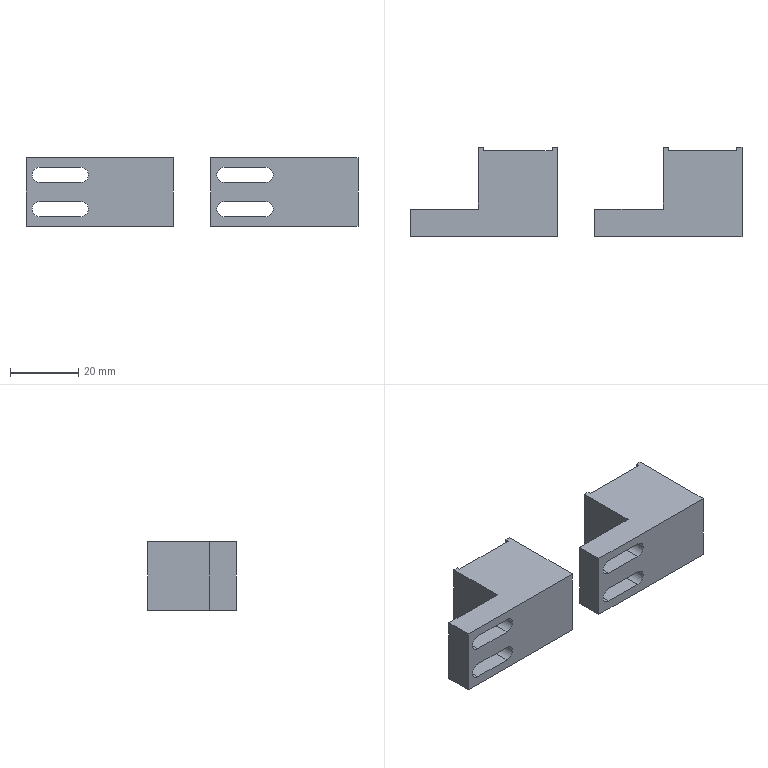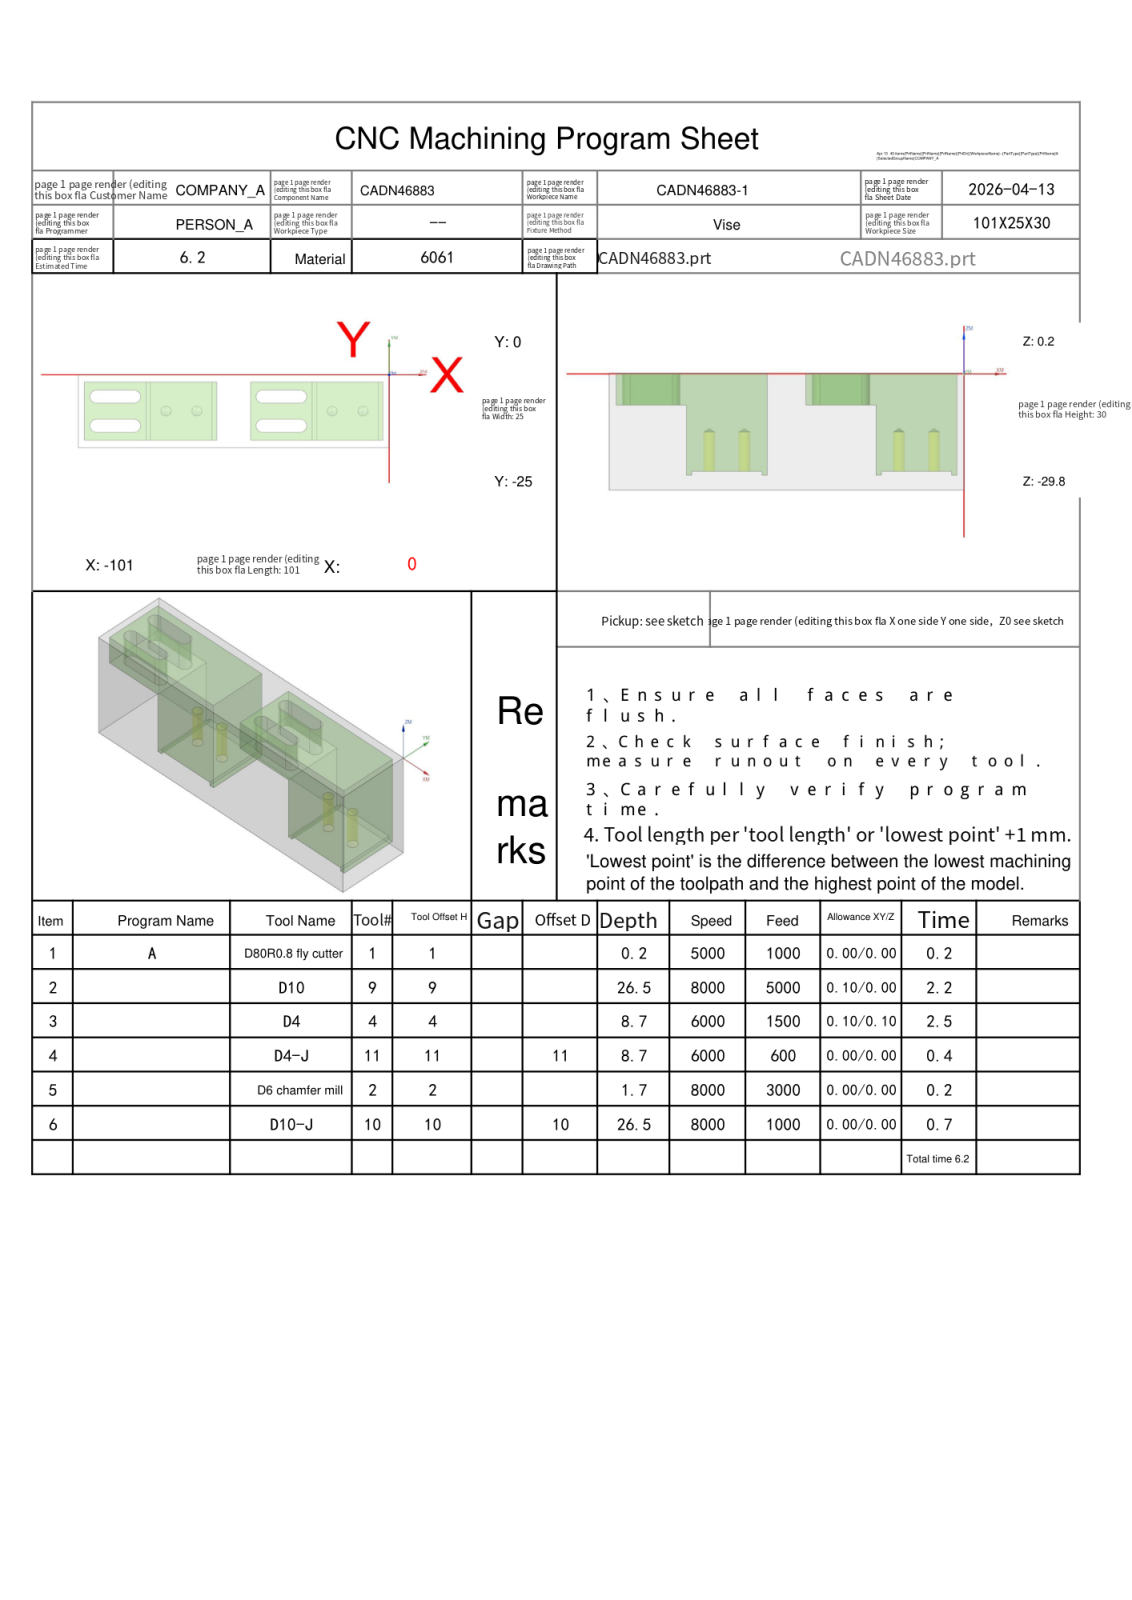NC program | NX | posted by the shop | part box 97 x 26 x 20 mm
Lines 1842 to 2082 of 2082:
N5 T02 M06
(D6 chamfer mill  D=6. R=0. H=02 ce=0.00 di=0.00)
(MAX_Z=20. MIN_Z=-1.5 Time=0.17M)
G00 G90 G54 X-77.25 Y-24.628 M03 S8000
G43 H02 Z20.
M08
Z2.099
G01 Z-1.5 F3000.
G03 X-77.17 Y-24.328 I-.52 J.3
X-77.47 Y-23.808 I-.6 J0.0
G01 X-77.5 Y-23.8
X-99.
G02 X-100.3 Y-22.5 I0.0 J1.3
G01 Y-2.5
G02 X-99. Y-1.2 I1.3 J0.0
G01 X-56.
G02 X-54.7 Y-2.5 I0.0 J-1.3
G01 Y-22.5
G02 X-56. Y-23.8 I-1.3 J0.0
G01 X-77.5
X-77.53 Y-23.808
G03 X-77.83 Y-24.328 I.3 J-.52
X-77.75 Y-24.628 I.6 J0.0
G01 Z2.099
G00 Z20.
X-89.25 Y-17.622
Z2.099
G01 Z-1.5
G03 X-89.33 Y-17.922 I.52 J-.3
X-89.03 Y-18.442 I.6 J0.0
G01 X-89. Y-18.45
X-83.
G03 X-82.05 Y-17.5 I0.0 J.95
X-82.177 Y-17.025 I-.95 J0.0
G01 X-82.328 Y-16.828
X-82.525 Y-16.677
X-82.754 Y-16.582
X-83. Y-16.55
X-95.
G03 X-95.95 Y-17.5 I0.0 J-.95
X-95.823 Y-17.975 I.95 J0.0
G01 X-95.672 Y-18.172
X-95.475 Y-18.323
X-95.246 Y-18.418
X-95. Y-18.45
X-89.
X-88.97 Y-18.442
G03 X-88.67 Y-17.922 I-.3 J.52
X-88.75 Y-17.622 I-.6 J0.0
G01 Z2.099
G00 Z6.
X-89.25 Y-7.622
Z2.099
G01 Z-1.5
G03 X-89.33 Y-7.922 I.52 J-.3
X-89.03 Y-8.442 I.6 J0.0
G01 X-89. Y-8.45
X-83.
G03 X-82.05 Y-7.5 I0.0 J.95
X-82.177 Y-7.025 I-.95 J0.0
G01 X-82.328 Y-6.828
X-82.525 Y-6.677
X-82.754 Y-6.582
X-83. Y-6.55
X-95.
G03 X-95.95 Y-7.5 I0.0 J-.95
X-95.823 Y-7.975 I.95 J0.0
G01 X-95.672 Y-8.172
X-95.475 Y-8.323
X-95.246 Y-8.418
X-95. Y-8.45
X-89.
X-88.97 Y-8.442
G03 X-88.67 Y-7.922 I-.3 J.52
X-88.75 Y-7.622 I-.6 J0.0
G01 Z2.099
G00 Z20.
X-23.25 Y-24.628
Z2.099
G01 Z-1.5
G03 X-23.17 Y-24.328 I-.52 J.3
X-23.47 Y-23.808 I-.6 J0.0
G01 X-23.5 Y-23.8
X-45.
G02 X-46.3 Y-22.5 I0.0 J1.3
G01 Y-2.5
G02 X-45. Y-1.2 I1.3 J0.0
G01 X-2.
G02 X-.7 Y-2.5 I0.0 J-1.3
G01 Y-22.5
G02 X-2. Y-23.8 I-1.3 J0.0
G01 X-23.5
X-23.53 Y-23.808
G03 X-23.83 Y-24.328 I.3 J-.52
X-23.75 Y-24.628 I.6 J0.0
G01 Z2.099
G00 Z20.
X-35.25 Y-17.622
Z2.099
G01 Z-1.5
G03 X-35.33 Y-17.922 I.52 J-.3
X-35.03 Y-18.442 I.6 J0.0
G01 X-35. Y-18.45
X-29.
G03 X-28.05 Y-17.5 I0.0 J.95
X-28.177 Y-17.025 I-.95 J0.0
G01 X-28.328 Y-16.828
X-28.525 Y-16.677
X-28.754 Y-16.582
X-29. Y-16.55
X-41.
G03 X-41.95 Y-17.5 I0.0 J-.95
X-41.823 Y-17.975 I.95 J0.0
G01 X-41.672 Y-18.172
X-41.475 Y-18.323
X-41.246 Y-18.418
X-41. Y-18.45
X-35.
X-34.97 Y-18.442
G03 X-34.67 Y-17.922 I-.3 J.52
X-34.75 Y-17.622 I-.6 J0.0
G01 Z2.099
G00 Z6.
Y-7.378
Z2.099
G01 Z-1.5
G03 X-34.67 Y-7.078 I-.52 J.3
X-34.97 Y-6.558 I-.6 J0.0
G01 X-35. Y-6.55
X-41.
G03 X-41.95 Y-7.5 I0.0 J-.95
X-41.823 Y-7.975 I.95 J0.0
G01 X-41.672 Y-8.172
X-41.475 Y-8.323
X-41.246 Y-8.418
X-41. Y-8.45
X-29.
G03 X-28.05 Y-7.5 I0.0 J.95
X-28.177 Y-7.025 I-.95 J0.0
G01 X-28.328 Y-6.828
X-28.525 Y-6.677
X-28.754 Y-6.582
X-29. Y-6.55
X-35.
X-35.03 Y-6.558
G03 X-35.33 Y-7.078 I.3 J-.52
X-35.25 Y-7.378 I.6 J0.0
G01 Z2.099
G00 Z20.
G91 G28 Z0.0
M05
M09
G91 G28 Z0.0
M01
N6 T10 M06
(D10-J  D=10. R=0. H=10 ce=0.00 di=0.00)
(D.N=10 MAX_Z=20. MIN_Z=-26.3 Time=0.68M)
G00 G90 G54 X-.987 Y-28.616 M03 S8000
G43 H10 Z20.
M08
Z-12.65
G01 Z-13.15 F1000.
G41 D10
X-1.003 Y-28.417
G03 X-2. Y-27.5 I-.997 J-.083
G01 X-45.
G02 X-50. Y-22.501 I0.0 J5.
G01 Y-2.5
G02 X-45. Y2.5 I5. J0.0
G01 X-2.
G02 X3. Y-2.5 I0.0 J-5.
G01 Y-22.5
G02 X-2. Y-27.5 I-5. J0.0
G01 X-2.5
G03 X-3.5 Y-28.5 I0.0 J-1.
G01 G40 Y-28.7
Z-12.65
G00 Z20.
X-76.5
Z-12.65
G01 Z-13.15
G41 D10
Y-28.5
G03 X-77.5 Y-27.5 I-1. J0.0
G01 X-99.
G02 X-104. Y-22.5 I0.0 J5.
G01 Y-2.5
G02 X-99. Y2.5 I5. J0.0
G01 X-56.
G02 X-51. Y-2.5 I0.0 J-5.
G01 Y-22.5
G02 X-56. Y-27.5 I-5. J0.0
G01 X-77.5
X-78.
G03 X-79. Y-28.5 I0.0 J-1.
G01 G40 Y-28.7
Z-12.65
G00 Z20.
X-54.987 Y-28.616
Z-25.8
G01 Z-26.3
G41 D10
X-55.003 Y-28.417
G03 X-56. Y-27.5 I-.997 J-.083
G01 X-99.
G02 X-104. Y-22.5 I0.0 J5.
G01 Y-2.5
G02 X-99. Y2.5 I5. J0.0
G01 X-56.
G02 X-51. Y-2.5 I0.0 J-5.
G01 Y-22.5
G02 X-56. Y-27.5 I-5. J0.0
G01 X-56.5
G03 X-57.5 Y-28.5 I0.0 J-1.
G01 G40 Y-28.7
X-50.149 Y-25.953
G41 D10
X-49.974 Y-25.856
G03 X-49.462 Y-24.983 I-.488 J.873
X-49.552 Y-24.569 I-1. J0.0
G02 X-50. Y-22.501 I4.552 J2.069
G01 Y-2.497
G02 X-45. Y2.5 I5. J-.003
G01 X-2.
G02 X3. Y-2.5 I0.0 J-5.
G01 Y-22.5
G02 X-2. Y-27.5 I-5. J0.0
G01 X-45.
G02 X-49.552 Y-24.569 I0.0 J5.
X-49.736 Y-24.104 I4.552 J2.069
G03 X-50.683 Y-23.425 I-.947 J-.321
X-51.004 Y-23.478 I0.0 J-1.
G01 G40 X-50.5 Y-24.898
Z-25.8
G00 Z20.
M05
M09
G91 G28 Z0.0
G91 G28 Y0.0
M30
%